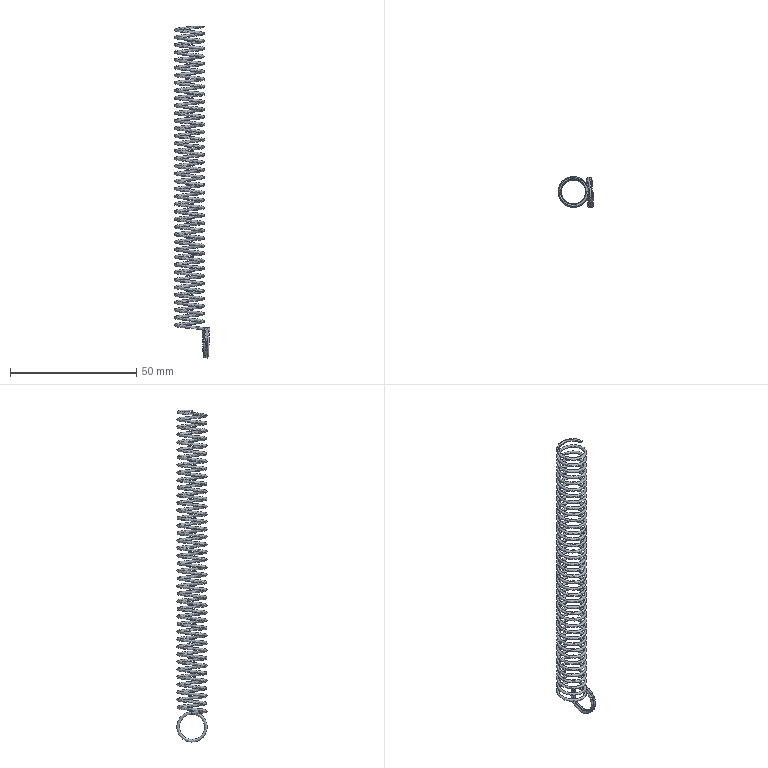Part | SolidWorks | features Helix 2, RefAxis 2, CompositeCurve 1, ICE 1, Sweep 1 | 1 solid | 6 faces | box 14.02 x 12 x 131.993 mm | volume 1022 mm3 | spline 3 | plane 3